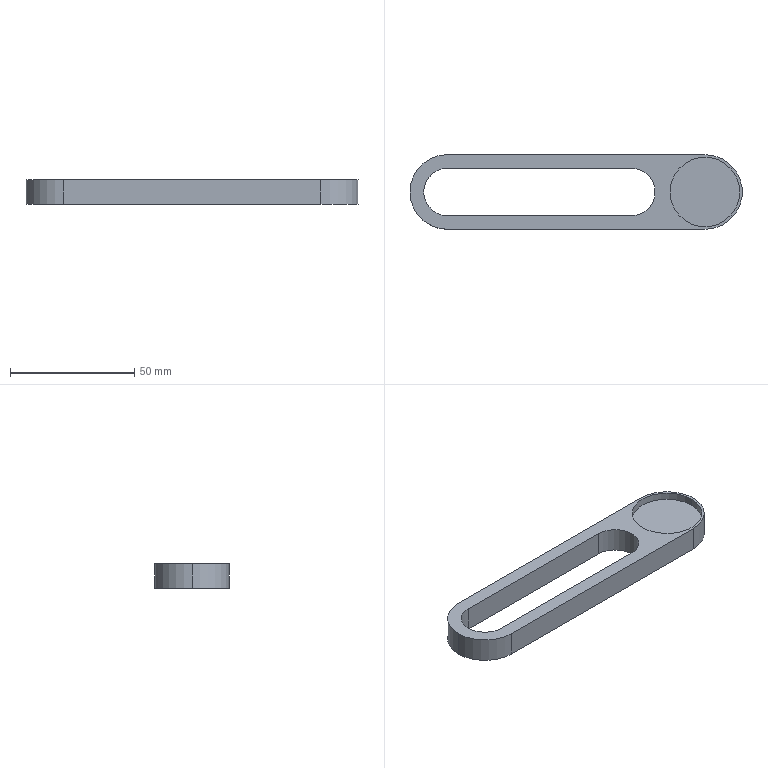Part | STEP file | PN_0040 | 1 solid | 15 faces | box 133.5 x 30 x 10 mm | volume 19376 mm3 | cylinder 8 | plane 7 | commonest cylinder face diameters 19 x3 30 x3 28 x2
STEP:
#1=CARTESIAN_POINT('',(0.,0.,0.));
#2=DIRECTION('',(0.,0.,1.));
#3=DIRECTION('',(1.,0.,0.));
#4=AXIS2_PLACEMENT_3D('',#1,#2,#3);
#5=CARTESIAN_POINT('',(117.5,0.,7.));
#6=VERTEX_POINT('',#5);
#7=CARTESIAN_POINT('',(117.5,0.,10.));
#8=VERTEX_POINT('',#7);
#9=CARTESIAN_POINT('',(117.5,0.,7.));
#10=DIRECTION('',(0.,0.,1.));
#11=VECTOR('',#10,1.);
#12=LINE('',#9,#11);
#13=CARTESIAN_POINT('',(103.5,0.,7.));
#14=DIRECTION('',(0.,0.,1.));
#15=DIRECTION('',(1.,0.,0.));
#16=AXIS2_PLACEMENT_3D('',#13,#14,#15);
#17=CYLINDRICAL_SURFACE('',#16,14.);
#18=CARTESIAN_POINT('',(6.283,0.));
#19=DIRECTION('',(0.,1.));
#20=VECTOR('',#19,1.);
#21=LINE('',#18,#20);
#22=(GEOMETRIC_REPRESENTATION_CONTEXT(2)PARAMETRIC_REPRESENTATION_CONTEXT()REPRESENTATION_CONTEXT('',''));
#23=DEFINITIONAL_REPRESENTATION('',(#21),#22);
#24=PCURVE('',#17,#23);
#25=CARTESIAN_POINT('',(103.5,0.,7.));
#26=DIRECTION('',(0.,0.,1.));
#27=DIRECTION('',(1.,0.,0.));
#28=AXIS2_PLACEMENT_3D('',#25,#26,#27);
#29=CYLINDRICAL_SURFACE('',#28,14.);
#30=CARTESIAN_POINT('',(0.,0.));
#31=DIRECTION('',(0.,1.));
#32=VECTOR('',#31,1.);
#33=LINE('',#30,#32);
#34=(GEOMETRIC_REPRESENTATION_CONTEXT(2)PARAMETRIC_REPRESENTATION_CONTEXT()REPRESENTATION_CONTEXT('',''));
#35=DEFINITIONAL_REPRESENTATION('',(#33),#34);
#36=PCURVE('',#29,#35);
#37=SURFACE_CURVE('',#12,(#24,#36),.PCURVE_S1.);
#38=EDGE_CURVE('',#6,#8,#37,.T.);
#39=ORIENTED_EDGE('',*,*,#38,.T.);
#40=CARTESIAN_POINT('',(89.5,0.,10.));
#41=VERTEX_POINT('',#40);
#42=CARTESIAN_POINT('',(103.5,0.,10.));
#43=DIRECTION('',(0.,0.,1.));
#44=DIRECTION('',(1.,0.,0.));
#45=AXIS2_PLACEMENT_3D('',#42,#43,#44);
#46=CIRCLE('',#45,14.);
#47=CARTESIAN_POINT('',(0.,3.));
#48=DIRECTION('',(1.,0.));
#49=VECTOR('',#48,1.);
#50=LINE('',#47,#49);
#51=(GEOMETRIC_REPRESENTATION_CONTEXT(2)PARAMETRIC_REPRESENTATION_CONTEXT()REPRESENTATION_CONTEXT('',''));
#52=DEFINITIONAL_REPRESENTATION('',(#50),#51);
#53=PCURVE('',#17,#52);
#54=CARTESIAN_POINT('',(0.,0.,10.));
#55=DIRECTION('',(0.,0.,1.));
#56=DIRECTION('',(1.,0.,0.));
#57=AXIS2_PLACEMENT_3D('',#54,#55,#56);
#58=PLANE('',#57);
#59=CARTESIAN_POINT('',(103.5,0.));
#60=DIRECTION('',(1.,0.));
#61=AXIS2_PLACEMENT_2D('',#59,#60);
#62=CIRCLE('',#61,14.);
#63=(GEOMETRIC_REPRESENTATION_CONTEXT(2)PARAMETRIC_REPRESENTATION_CONTEXT()REPRESENTATION_CONTEXT('',''));
#64=DEFINITIONAL_REPRESENTATION('',(#62),#63);
#65=PCURVE('',#58,#64);
#66=SURFACE_CURVE('',#46,(#53,#65),.PCURVE_S1.);
#67=EDGE_CURVE('',#41,#8,#66,.T.);
#68=ORIENTED_EDGE('',*,*,#67,.F.);
#69=CARTESIAN_POINT('',(89.5,0.,7.));
#70=VERTEX_POINT('',#69);
#71=CARTESIAN_POINT('',(89.5,0.,7.));
#72=DIRECTION('',(0.,0.,1.));
#73=VECTOR('',#72,1.);
#74=LINE('',#71,#73);
#75=CARTESIAN_POINT('',(3.142,0.));
#76=DIRECTION('',(0.,1.));
#77=VECTOR('',#76,1.);
#78=LINE('',#75,#77);
#79=(GEOMETRIC_REPRESENTATION_CONTEXT(2)PARAMETRIC_REPRESENTATION_CONTEXT()REPRESENTATION_CONTEXT('',''));
#80=DEFINITIONAL_REPRESENTATION('',(#78),#79);
#81=PCURVE('',#17,#80);
#82=CARTESIAN_POINT('',(3.142,0.));
#83=DIRECTION('',(0.,1.));
#84=VECTOR('',#83,1.);
#85=LINE('',#82,#84);
#86=(GEOMETRIC_REPRESENTATION_CONTEXT(2)PARAMETRIC_REPRESENTATION_CONTEXT()REPRESENTATION_CONTEXT('',''));
#87=DEFINITIONAL_REPRESENTATION('',(#85),#86);
#88=PCURVE('',#29,#87);
#89=SURFACE_CURVE('',#74,(#81,#88),.PCURVE_S1.);
#90=EDGE_CURVE('',#70,#41,#89,.T.);
#91=ORIENTED_EDGE('',*,*,#90,.F.);
#92=CARTESIAN_POINT('',(103.5,0.,7.));
#93=DIRECTION('',(0.,0.,1.));
#94=DIRECTION('',(1.,0.,0.));
#95=AXIS2_PLACEMENT_3D('',#92,#93,#94);
#96=CIRCLE('',#95,14.);
#97=CARTESIAN_POINT('',(0.,0.));
#98=DIRECTION('',(1.,0.));
#99=VECTOR('',#98,1.);
#100=LINE('',#97,#99);
#101=(GEOMETRIC_REPRESENTATION_CONTEXT(2)PARAMETRIC_REPRESENTATION_CONTEXT()REPRESENTATION_CONTEXT('',''));
#102=DEFINITIONAL_REPRESENTATION('',(#100),#101);
#103=PCURVE('',#17,#102);
#104=CARTESIAN_POINT('',(103.5,0.,7.));
#105=DIRECTION('',(0.,0.,1.));
#106=DIRECTION('',(1.,0.,0.));
#107=AXIS2_PLACEMENT_3D('',#104,#105,#106);
#108=PLANE('',#107);
#109=CARTESIAN_POINT('',(0.,0.));
#110=DIRECTION('',(1.,0.));
#111=AXIS2_PLACEMENT_2D('',#109,#110);
#112=CIRCLE('',#111,14.);
#113=(GEOMETRIC_REPRESENTATION_CONTEXT(2)PARAMETRIC_REPRESENTATION_CONTEXT()REPRESENTATION_CONTEXT('',''));
#114=DEFINITIONAL_REPRESENTATION('',(#112),#113);
#115=PCURVE('',#108,#114);
#116=SURFACE_CURVE('',#96,(#103,#115),.PCURVE_S1.);
#117=EDGE_CURVE('',#70,#6,#116,.T.);
#118=ORIENTED_EDGE('',*,*,#117,.T.);
#119=EDGE_LOOP('',(#39,#68,#91,#118));
#120=FACE_BOUND('',#119,.F.);
#121=ADVANCED_FACE('',(#120),#17,.F.);
#122=CARTESIAN_POINT('',(0.,9.5,10.));
#123=VERTEX_POINT('',#122);
#124=CARTESIAN_POINT('',(0.,9.5,0.));
#125=VERTEX_POINT('',#124);
#126=CARTESIAN_POINT('',(0.,9.5,10.));
#127=DIRECTION('',(0.,0.,-1.));
#128=VECTOR('',#127,1.);
#129=LINE('',#126,#128);
#130=CARTESIAN_POINT('',(0.,0.,10.));
#131=DIRECTION('',(0.,0.,-1.));
#132=DIRECTION('',(-1.,0.,0.));
#133=AXIS2_PLACEMENT_3D('',#130,#131,#132);
#134=CYLINDRICAL_SURFACE('',#133,9.5);
#135=CARTESIAN_POINT('',(1.571,0.));
#136=DIRECTION('',(0.,1.));
#137=VECTOR('',#136,1.);
#138=LINE('',#135,#137);
#139=(GEOMETRIC_REPRESENTATION_CONTEXT(2)PARAMETRIC_REPRESENTATION_CONTEXT()REPRESENTATION_CONTEXT('',''));
#140=DEFINITIONAL_REPRESENTATION('',(#138),#139);
#141=PCURVE('',#134,#140);
#142=CARTESIAN_POINT('',(0.,9.5,10.));
#143=DIRECTION('',(0.,-1.,0.));
#144=DIRECTION('',(0.,0.,-1.));
#145=AXIS2_PLACEMENT_3D('',#142,#143,#144);
#146=PLANE('',#145);
#147=CARTESIAN_POINT('',(0.,0.));
#148=DIRECTION('',(1.,0.));
#149=VECTOR('',#148,1.);
#150=LINE('',#147,#149);
#151=(GEOMETRIC_REPRESENTATION_CONTEXT(2)PARAMETRIC_REPRESENTATION_CONTEXT()REPRESENTATION_CONTEXT('',''));
#152=DEFINITIONAL_REPRESENTATION('',(#150),#151);
#153=PCURVE('',#146,#152);
#154=SURFACE_CURVE('',#129,(#141,#153),.PCURVE_S1.);
#155=EDGE_CURVE('',#123,#125,#154,.T.);
#156=ORIENTED_EDGE('',*,*,#155,.T.);
#157=CARTESIAN_POINT('',(-9.5,0.,0.));
#158=VERTEX_POINT('',#157);
#159=CARTESIAN_POINT('',(0.,0.,0.));
#160=DIRECTION('',(0.,0.,1.));
#161=DIRECTION('',(1.,0.,0.));
#162=AXIS2_PLACEMENT_3D('',#159,#160,#161);
#163=CIRCLE('',#162,9.5);
#164=CARTESIAN_POINT('',(3.142,10.));
#165=DIRECTION('',(-1.,0.));
#166=VECTOR('',#165,1.);
#167=LINE('',#164,#166);
#168=(GEOMETRIC_REPRESENTATION_CONTEXT(2)PARAMETRIC_REPRESENTATION_CONTEXT()REPRESENTATION_CONTEXT('',''));
#169=DEFINITIONAL_REPRESENTATION('',(#167),#168);
#170=PCURVE('',#134,#169);
#171=CARTESIAN_POINT('',(0.,0.,0.));
#172=DIRECTION('',(0.,0.,1.));
#173=DIRECTION('',(1.,0.,0.));
#174=AXIS2_PLACEMENT_3D('',#171,#172,#173);
#175=PLANE('',#174);
#176=CARTESIAN_POINT('',(0.,0.));
#177=DIRECTION('',(1.,0.));
#178=AXIS2_PLACEMENT_2D('',#176,#177);
#179=CIRCLE('',#178,9.5);
#180=(GEOMETRIC_REPRESENTATION_CONTEXT(2)PARAMETRIC_REPRESENTATION_CONTEXT()REPRESENTATION_CONTEXT('',''));
#181=DEFINITIONAL_REPRESENTATION('',(#179),#180);
#182=PCURVE('',#175,#181);
#183=SURFACE_CURVE('',#163,(#170,#182),.PCURVE_S1.);
#184=EDGE_CURVE('',#125,#158,#183,.T.);
#185=ORIENTED_EDGE('',*,*,#184,.T.);
#186=CARTESIAN_POINT('',(-9.5,0.,10.));
#187=VERTEX_POINT('',#186);
#188=CARTESIAN_POINT('',(-9.5,0.,10.));
#189=DIRECTION('',(0.,0.,-1.));
#190=VECTOR('',#189,1.);
#191=LINE('',#188,#190);
#192=CARTESIAN_POINT('',(0.,0.));
#193=DIRECTION('',(0.,1.));
#194=VECTOR('',#193,1.);
#195=LINE('',#192,#194);
#196=(GEOMETRIC_REPRESENTATION_CONTEXT(2)PARAMETRIC_REPRESENTATION_CONTEXT()REPRESENTATION_CONTEXT('',''));
#197=DEFINITIONAL_REPRESENTATION('',(#195),#196);
#198=PCURVE('',#134,#197);
#199=CARTESIAN_POINT('',(0.,0.,10.));
#200=DIRECTION('',(0.,0.,-1.));
#201=DIRECTION('',(-1.,0.,0.));
#202=AXIS2_PLACEMENT_3D('',#199,#200,#201);
#203=CYLINDRICAL_SURFACE('',#202,9.5);
#204=CARTESIAN_POINT('',(6.283,0.));
#205=DIRECTION('',(0.,1.));
#206=VECTOR('',#205,1.);
#207=LINE('',#204,#206);
#208=(GEOMETRIC_REPRESENTATION_CONTEXT(2)PARAMETRIC_REPRESENTATION_CONTEXT()REPRESENTATION_CONTEXT('',''));
#209=DEFINITIONAL_REPRESENTATION('',(#207),#208);
#210=PCURVE('',#203,#209);
#211=SURFACE_CURVE('',#191,(#198,#210),.PCURVE_S1.);
#212=EDGE_CURVE('',#187,#158,#211,.T.);
#213=ORIENTED_EDGE('',*,*,#212,.F.);
#214=CARTESIAN_POINT('',(0.,0.,10.));
#215=DIRECTION('',(0.,0.,1.));
#216=DIRECTION('',(1.,0.,0.));
#217=AXIS2_PLACEMENT_3D('',#214,#215,#216);
#218=CIRCLE('',#217,9.5);
#219=CARTESIAN_POINT('',(3.142,0.));
#220=DIRECTION('',(-1.,0.));
#221=VECTOR('',#220,1.);
#222=LINE('',#219,#221);
#223=(GEOMETRIC_REPRESENTATION_CONTEXT(2)PARAMETRIC_REPRESENTATION_CONTEXT()REPRESENTATION_CONTEXT('',''));
#224=DEFINITIONAL_REPRESENTATION('',(#222),#223);
#225=PCURVE('',#134,#224);
#226=CARTESIAN_POINT('',(0.,0.));
#227=DIRECTION('',(1.,0.));
#228=AXIS2_PLACEMENT_2D('',#226,#227);
#229=CIRCLE('',#228,9.5);
#230=(GEOMETRIC_REPRESENTATION_CONTEXT(2)PARAMETRIC_REPRESENTATION_CONTEXT()REPRESENTATION_CONTEXT('',''));
#231=DEFINITIONAL_REPRESENTATION('',(#229),#230);
#232=PCURVE('',#58,#231);
#233=SURFACE_CURVE('',#218,(#225,#232),.PCURVE_S1.);
#234=EDGE_CURVE('',#123,#187,#233,.T.);
#235=ORIENTED_EDGE('',*,*,#234,.F.);
#236=EDGE_LOOP('',(#156,#185,#213,#235));
#237=FACE_BOUND('',#236,.F.);
#238=ADVANCED_FACE('',(#237),#134,.F.);
#239=CARTESIAN_POINT('',(-15.,0.,10.));
#240=VERTEX_POINT('',#239);
#241=CARTESIAN_POINT('',(0.,-15.,10.));
#242=VERTEX_POINT('',#241);
#243=CARTESIAN_POINT('',(0.,0.,10.));
#244=DIRECTION('',(0.,0.,1.));
#245=DIRECTION('',(1.,0.,0.));
#246=AXIS2_PLACEMENT_3D('',#243,#244,#245);
#247=CIRCLE('',#246,15.);
#248=CARTESIAN_POINT('',(0.,0.,10.));
#249=DIRECTION('',(0.,0.,-1.));
#250=DIRECTION('',(-1.,0.,0.));
#251=AXIS2_PLACEMENT_3D('',#248,#249,#250);
#252=CYLINDRICAL_SURFACE('',#251,15.);
#253=CARTESIAN_POINT('',(9.425,0.));
#254=DIRECTION('',(-1.,0.));
#255=VECTOR('',#254,1.);
#256=LINE('',#253,#255);
#257=(GEOMETRIC_REPRESENTATION_CONTEXT(2)PARAMETRIC_REPRESENTATION_CONTEXT()REPRESENTATION_CONTEXT('',''));
#258=DEFINITIONAL_REPRESENTATION('',(#256),#257);
#259=PCURVE('',#252,#258);
#260=CARTESIAN_POINT('',(0.,0.));
#261=DIRECTION('',(1.,0.));
#262=AXIS2_PLACEMENT_2D('',#260,#261);
#263=CIRCLE('',#262,15.);
#264=(GEOMETRIC_REPRESENTATION_CONTEXT(2)PARAMETRIC_REPRESENTATION_CONTEXT()REPRESENTATION_CONTEXT('',''));
#265=DEFINITIONAL_REPRESENTATION('',(#263),#264);
#266=PCURVE('',#58,#265);
#267=SURFACE_CURVE('',#247,(#259,#266),.PCURVE_S1.);
#268=EDGE_CURVE('',#240,#242,#267,.T.);
#269=ORIENTED_EDGE('',*,*,#268,.F.);
#270=CARTESIAN_POINT('',(-15.,0.,0.));
#271=VERTEX_POINT('',#270);
#272=CARTESIAN_POINT('',(-15.,0.,10.));
#273=DIRECTION('',(0.,0.,-1.));
#274=VECTOR('',#273,1.);
#275=LINE('',#272,#274);
#276=CARTESIAN_POINT('',(6.283,0.));
#277=DIRECTION('',(0.,1.));
#278=VECTOR('',#277,1.);
#279=LINE('',#276,#278);
#280=(GEOMETRIC_REPRESENTATION_CONTEXT(2)PARAMETRIC_REPRESENTATION_CONTEXT()REPRESENTATION_CONTEXT('',''));
#281=DEFINITIONAL_REPRESENTATION('',(#279),#280);
#282=PCURVE('',#252,#281);
#283=CARTESIAN_POINT('',(0.,0.,10.));
#284=DIRECTION('',(0.,0.,-1.));
#285=DIRECTION('',(-1.,0.,0.));
#286=AXIS2_PLACEMENT_3D('',#283,#284,#285);
#287=CYLINDRICAL_SURFACE('',#286,15.);
#288=CARTESIAN_POINT('',(0.,0.));
#289=DIRECTION('',(0.,1.));
#290=VECTOR('',#289,1.);
#291=LINE('',#288,#290);
#292=(GEOMETRIC_REPRESENTATION_CONTEXT(2)PARAMETRIC_REPRESENTATION_CONTEXT()REPRESENTATION_CONTEXT('',''));
#293=DEFINITIONAL_REPRESENTATION('',(#291),#292);
#294=PCURVE('',#287,#293);
#295=SURFACE_CURVE('',#275,(#282,#294),.PCURVE_S1.);
#296=EDGE_CURVE('',#240,#271,#295,.T.);
#297=ORIENTED_EDGE('',*,*,#296,.T.);
#298=CARTESIAN_POINT('',(0.,-15.,0.));
#299=VERTEX_POINT('',#298);
#300=CARTESIAN_POINT('',(0.,0.,0.));
#301=DIRECTION('',(0.,0.,1.));
#302=DIRECTION('',(1.,0.,0.));
#303=AXIS2_PLACEMENT_3D('',#300,#301,#302);
#304=CIRCLE('',#303,15.);
#305=CARTESIAN_POINT('',(9.425,10.));
#306=DIRECTION('',(-1.,0.));
#307=VECTOR('',#306,1.);
#308=LINE('',#305,#307);
#309=(GEOMETRIC_REPRESENTATION_CONTEXT(2)PARAMETRIC_REPRESENTATION_CONTEXT()REPRESENTATION_CONTEXT('',''));
#310=DEFINITIONAL_REPRESENTATION('',(#308),#309);
#311=PCURVE('',#252,#310);
#312=CARTESIAN_POINT('',(0.,0.));
#313=DIRECTION('',(1.,0.));
#314=AXIS2_PLACEMENT_2D('',#312,#313);
#315=CIRCLE('',#314,15.);
#316=(GEOMETRIC_REPRESENTATION_CONTEXT(2)PARAMETRIC_REPRESENTATION_CONTEXT()REPRESENTATION_CONTEXT('',''));
#317=DEFINITIONAL_REPRESENTATION('',(#315),#316);
#318=PCURVE('',#175,#317);
#319=SURFACE_CURVE('',#304,(#311,#318),.PCURVE_S1.);
#320=EDGE_CURVE('',#271,#299,#319,.T.);
#321=ORIENTED_EDGE('',*,*,#320,.T.);
#322=CARTESIAN_POINT('',(0.,-15.,10.));
#323=DIRECTION('',(0.,0.,-1.));
#324=VECTOR('',#323,1.);
#325=LINE('',#322,#324);
#326=CARTESIAN_POINT('',(4.712,0.));
#327=DIRECTION('',(0.,1.));
#328=VECTOR('',#327,1.);
#329=LINE('',#326,#328);
#330=(GEOMETRIC_REPRESENTATION_CONTEXT(2)PARAMETRIC_REPRESENTATION_CONTEXT()REPRESENTATION_CONTEXT('',''));
#331=DEFINITIONAL_REPRESENTATION('',(#329),#330);
#332=PCURVE('',#252,#331);
#333=CARTESIAN_POINT('',(0.,-15.,10.));
#334=DIRECTION('',(0.,1.,0.));
#335=DIRECTION('',(-1.,0.,0.));
#336=AXIS2_PLACEMENT_3D('',#333,#334,#335);
#337=PLANE('',#336);
#338=CARTESIAN_POINT('',(0.,0.));
#339=DIRECTION('',(0.,-1.));
#340=VECTOR('',#339,1.);
#341=LINE('',#338,#340);
#342=(GEOMETRIC_REPRESENTATION_CONTEXT(2)PARAMETRIC_REPRESENTATION_CONTEXT()REPRESENTATION_CONTEXT('',''));
#343=DEFINITIONAL_REPRESENTATION('',(#341),#342);
#344=PCURVE('',#337,#343);
#345=SURFACE_CURVE('',#325,(#332,#344),.PCURVE_S1.);
#346=EDGE_CURVE('',#242,#299,#345,.T.);
#347=ORIENTED_EDGE('',*,*,#346,.F.);
#348=EDGE_LOOP('',(#269,#297,#321,#347));
#349=FACE_BOUND('',#348,.T.);
#350=ADVANCED_FACE('',(#349),#252,.T.);
#351=CARTESIAN_POINT('',(103.5,0.,10.));
#352=DIRECTION('',(0.,0.,1.));
#353=DIRECTION('',(1.,0.,0.));
#354=AXIS2_PLACEMENT_3D('',#351,#352,#353);
#355=CIRCLE('',#354,14.);
#356=CARTESIAN_POINT('',(103.5,0.));
#357=DIRECTION('',(1.,0.));
#358=AXIS2_PLACEMENT_2D('',#356,#357);
#359=CIRCLE('',#358,14.);
#360=(GEOMETRIC_REPRESENTATION_CONTEXT(2)PARAMETRIC_REPRESENTATION_CONTEXT()REPRESENTATION_CONTEXT('',''));
#361=DEFINITIONAL_REPRESENTATION('',(#359),#360);
#362=PCURVE('',#58,#361);
#363=CARTESIAN_POINT('',(0.,3.));
#364=DIRECTION('',(1.,0.));
#365=VECTOR('',#364,1.);
#366=LINE('',#363,#365);
#367=(GEOMETRIC_REPRESENTATION_CONTEXT(2)PARAMETRIC_REPRESENTATION_CONTEXT()REPRESENTATION_CONTEXT('',''));
#368=DEFINITIONAL_REPRESENTATION('',(#366),#367);
#369=PCURVE('',#29,#368);
#370=SURFACE_CURVE('',#355,(#362,#369),.PCURVE_S1.);
#371=EDGE_CURVE('',#8,#41,#370,.T.);
#372=ORIENTED_EDGE('',*,*,#371,.F.);
#373=ORIENTED_EDGE('',*,*,#67,.F.);
#374=EDGE_LOOP('',(#372,#373));
#375=FACE_BOUND('',#374,.T.);
#376=CARTESIAN_POINT('',(0.,15.,10.));
#377=VERTEX_POINT('',#376);
#378=CARTESIAN_POINT('',(0.,0.,10.));
#379=DIRECTION('',(0.,0.,1.));
#380=DIRECTION('',(1.,0.,0.));
#381=AXIS2_PLACEMENT_3D('',#378,#379,#380);
#382=CIRCLE('',#381,15.);
#383=CARTESIAN_POINT('',(0.,0.));
#384=DIRECTION('',(1.,0.));
#385=AXIS2_PLACEMENT_2D('',#383,#384);
#386=CIRCLE('',#385,15.);
#387=(GEOMETRIC_REPRESENTATION_CONTEXT(2)PARAMETRIC_REPRESENTATION_CONTEXT()REPRESENTATION_CONTEXT('',''));
#388=DEFINITIONAL_REPRESENTATION('',(#386),#387);
#389=PCURVE('',#58,#388);
#390=CARTESIAN_POINT('',(3.142,0.));
#391=DIRECTION('',(-1.,0.));
#392=VECTOR('',#391,1.);
#393=LINE('',#390,#392);
#394=(GEOMETRIC_REPRESENTATION_CONTEXT(2)PARAMETRIC_REPRESENTATION_CONTEXT()REPRESENTATION_CONTEXT('',''));
#395=DEFINITIONAL_REPRESENTATION('',(#393),#394);
#396=PCURVE('',#287,#395);
#397=SURFACE_CURVE('',#382,(#389,#396),.PCURVE_S1.);
#398=EDGE_CURVE('',#377,#240,#397,.T.);
#399=ORIENTED_EDGE('',*,*,#398,.T.);
#400=ORIENTED_EDGE('',*,*,#268,.T.);
#401=CARTESIAN_POINT('',(103.5,-15.,10.));
#402=VERTEX_POINT('',#401);
#403=CARTESIAN_POINT('',(0.,-15.,10.));
#404=DIRECTION('',(1.,0.,0.));
#405=VECTOR('',#404,1.);
#406=LINE('',#403,#405);
#407=CARTESIAN_POINT('',(0.,-15.));
#408=DIRECTION('',(1.,0.));
#409=VECTOR('',#408,1.);
#410=LINE('',#407,#409);
#411=(GEOMETRIC_REPRESENTATION_CONTEXT(2)PARAMETRIC_REPRESENTATION_CONTEXT()REPRESENTATION_CONTEXT('',''));
#412=DEFINITIONAL_REPRESENTATION('',(#410),#411);
#413=PCURVE('',#58,#412);
#414=CARTESIAN_POINT('',(0.,0.));
#415=DIRECTION('',(-1.,0.));
#416=VECTOR('',#415,1.);
#417=LINE('',#414,#416);
#418=(GEOMETRIC_REPRESENTATION_CONTEXT(2)PARAMETRIC_REPRESENTATION_CONTEXT()REPRESENTATION_CONTEXT('',''));
#419=DEFINITIONAL_REPRESENTATION('',(#417),#418);
#420=PCURVE('',#337,#419);
#421=SURFACE_CURVE('',#406,(#413,#420),.PCURVE_S1.);
#422=EDGE_CURVE('',#242,#402,#421,.T.);
#423=ORIENTED_EDGE('',*,*,#422,.T.);
#424=CARTESIAN_POINT('',(103.5,15.,10.));
#425=VERTEX_POINT('',#424);
#426=CARTESIAN_POINT('',(103.5,0.,10.));
#427=DIRECTION('',(0.,0.,1.));
#428=DIRECTION('',(1.,0.,0.));
#429=AXIS2_PLACEMENT_3D('',#426,#427,#428);
#430=CIRCLE('',#429,15.);
#431=CARTESIAN_POINT('',(103.5,0.));
#432=DIRECTION('',(1.,0.));
#433=AXIS2_PLACEMENT_2D('',#431,#432);
#434=CIRCLE('',#433,15.);
#435=(GEOMETRIC_REPRESENTATION_CONTEXT(2)PARAMETRIC_REPRESENTATION_CONTEXT()REPRESENTATION_CONTEXT('',''));
#436=DEFINITIONAL_REPRESENTATION('',(#434),#435);
#437=PCURVE('',#58,#436);
#438=CARTESIAN_POINT('',(103.5,0.,10.));
#439=DIRECTION('',(0.,0.,-1.));
#440=DIRECTION('',(-1.,0.,0.));
#441=AXIS2_PLACEMENT_3D('',#438,#439,#440);
#442=CYLINDRICAL_SURFACE('',#441,15.);
#443=CARTESIAN_POINT('',(9.425,0.));
#444=DIRECTION('',(-1.,0.));
#445=VECTOR('',#444,1.);
#446=LINE('',#443,#445);
#447=(GEOMETRIC_REPRESENTATION_CONTEXT(2)PARAMETRIC_REPRESENTATION_CONTEXT()REPRESENTATION_CONTEXT('',''));
#448=DEFINITIONAL_REPRESENTATION('',(#446),#447);
#449=PCURVE('',#442,#448);
#450=SURFACE_CURVE('',#430,(#437,#449),.PCURVE_S1.);
#451=EDGE_CURVE('',#402,#425,#450,.T.);
#452=ORIENTED_EDGE('',*,*,#451,.T.);
#453=CARTESIAN_POINT('',(0.,15.,10.));
#454=DIRECTION('',(-1.,0.,0.));
#455=VECTOR('',#454,1.);
#456=LINE('',#453,#455);
#457=CARTESIAN_POINT('',(0.,15.));
#458=DIRECTION('',(-1.,0.));
#459=VECTOR('',#458,1.);
#460=LINE('',#457,#459);
#461=(GEOMETRIC_REPRESENTATION_CONTEXT(2)PARAMETRIC_REPRESENTATION_CONTEXT()REPRESENTATION_CONTEXT('',''));
#462=DEFINITIONAL_REPRESENTATION('',(#460),#461);
#463=PCURVE('',#58,#462);
#464=CARTESIAN_POINT('',(0.,15.,10.));
#465=DIRECTION('',(0.,-1.,0.));
#466=DIRECTION('',(0.,0.,-1.));
#467=AXIS2_PLACEMENT_3D('',#464,#465,#466);
#468=PLANE('',#467);
#469=CARTESIAN_POINT('',(0.,0.));
#470=DIRECTION('',(0.,-1.));
#471=VECTOR('',#470,1.);
#472=LINE('',#469,#471);
#473=(GEOMETRIC_REPRESENTATION_CONTEXT(2)PARAMETRIC_REPRESENTATION_CONTEXT()REPRESENTATION_CONTEXT('',''));
#474=DEFINITIONAL_REPRESENTATION('',(#472),#473);
#475=PCURVE('',#468,#474);
#476=SURFACE_CURVE('',#456,(#463,#475),.PCURVE_S1.);
#477=EDGE_CURVE('',#425,#377,#476,.T.);
#478=ORIENTED_EDGE('',*,*,#477,.T.);
#479=EDGE_LOOP('',(#399,#400,#423,#452,#478));
#480=FACE_BOUND('',#479,.T.);
#481=CARTESIAN_POINT('',(0.,-9.5,10.));
#482=VERTEX_POINT('',#481);
#483=CARTESIAN_POINT('',(74.,-9.5,10.));
#484=VERTEX_POINT('',#483);
#485=CARTESIAN_POINT('',(0.,-9.5,10.));
#486=DIRECTION('',(1.,0.,0.));
#487=VECTOR('',#486,1.);
#488=LINE('',#485,#487);
#489=CARTESIAN_POINT('',(0.,-9.5));
#490=DIRECTION('',(1.,0.));
#491=VECTOR('',#490,1.);
#492=LINE('',#489,#491);
#493=(GEOMETRIC_REPRESENTATION_CONTEXT(2)PARAMETRIC_REPRESENTATION_CONTEXT()REPRESENTATION_CONTEXT('',''));
#494=DEFINITIONAL_REPRESENTATION('',(#492),#493);
#495=PCURVE('',#58,#494);
#496=CARTESIAN_POINT('',(0.,-9.5,10.));
#497=DIRECTION('',(0.,1.,0.));
#498=DIRECTION('',(-1.,0.,0.));
#499=AXIS2_PLACEMENT_3D('',#496,#497,#498);
#500=PLANE('',#499);
#501=CARTESIAN_POINT('',(0.,0.));
#502=DIRECTION('',(-1.,0.));
#503=VECTOR('',#502,1.);
#504=LINE('',#501,#503);
#505=(GEOMETRIC_REPRESENTATION_CONTEXT(2)PARAMETRIC_REPRESENTATION_CONTEXT()REPRESENTATION_CONTEXT('',''));
#506=DEFINITIONAL_REPRESENTATION('',(#504),#505);
#507=PCURVE('',#500,#506);
#508=SURFACE_CURVE('',#488,(#495,#507),.PCURVE_S1.);
#509=EDGE_CURVE('',#482,#484,#508,.T.);
#510=ORIENTED_EDGE('',*,*,#509,.F.);
#511=CARTESIAN_POINT('',(0.,0.,10.));
#512=DIRECTION('',(0.,0.,1.));
#513=DIRECTION('',(1.,0.,0.));
#514=AXIS2_PLACEMENT_3D('',#511,#512,#513);
#515=CIRCLE('',#514,9.5);
#516=CARTESIAN_POINT('',(0.,0.));
#517=DIRECTION('',(1.,0.));
#518=AXIS2_PLACEMENT_2D('',#516,#517);
#519=CIRCLE('',#518,9.5);
#520=(GEOMETRIC_REPRESENTATION_CONTEXT(2)PARAMETRIC_REPRESENTATION_CONTEXT()REPRESENTATION_CONTEXT('',''));
#521=DEFINITIONAL_REPRESENTATION('',(#519),#520);
#522=PCURVE('',#58,#521);
#523=CARTESIAN_POINT('',(9.425,0.));
#524=DIRECTION('',(-1.,0.));
#525=VECTOR('',#524,1.);
#526=LINE('',#523,#525);
#527=(GEOMETRIC_REPRESENTATION_CONTEXT(2)PARAMETRIC_REPRESENTATION_CONTEXT()REPRESENTATION_CONTEXT('',''));
#528=DEFINITIONAL_REPRESENTATION('',(#526),#527);
#529=PCURVE('',#203,#528);
#530=SURFACE_CURVE('',#515,(#522,#529),.PCURVE_S1.);
#531=EDGE_CURVE('',#187,#482,#530,.T.);
#532=ORIENTED_EDGE('',*,*,#531,.F.);
#533=ORIENTED_EDGE('',*,*,#234,.F.);
#534=CARTESIAN_POINT('',(74.,9.5,10.));
#535=VERTEX_POINT('',#534);
#536=CARTESIAN_POINT('',(0.,9.5,10.));
#537=DIRECTION('',(-1.,0.,0.));
#538=VECTOR('',#537,1.);
#539=LINE('',#536,#538);
#540=CARTESIAN_POINT('',(0.,9.5));
#541=DIRECTION('',(-1.,0.));
#542=VECTOR('',#541,1.);
#543=LINE('',#540,#542);
#544=(GEOMETRIC_REPRESENTATION_CONTEXT(2)PARAMETRIC_REPRESENTATION_CONTEXT()REPRESENTATION_CONTEXT('',''));
#545=DEFINITIONAL_REPRESENTATION('',(#543),#544);
#546=PCURVE('',#58,#545);
#547=CARTESIAN_POINT('',(0.,0.));
#548=DIRECTION('',(0.,-1.));
#549=VECTOR('',#548,1.);
#550=LINE('',#547,#549);
#551=(GEOMETRIC_REPRESENTATION_CONTEXT(2)PARAMETRIC_REPRESENTATION_CONTEXT()REPRESENTATION_CONTEXT('',''));
#552=DEFINITIONAL_REPRESENTATION('',(#550),#551);
#553=PCURVE('',#146,#552);
#554=SURFACE_CURVE('',#539,(#546,#553),.PCURVE_S1.);
#555=EDGE_CURVE('',#535,#123,#554,.T.);
#556=ORIENTED_EDGE('',*,*,#555,.F.);
#557=CARTESIAN_POINT('',(74.,0.,10.));
#558=DIRECTION('',(0.,0.,1.));
#559=DIRECTION('',(1.,0.,0.));
#560=AXIS2_PLACEMENT_3D('',#557,#558,#559);
#561=CIRCLE('',#560,9.5);
#562=CARTESIAN_POINT('',(74.,0.));
#563=DIRECTION('',(1.,0.));
#564=AXIS2_PLACEMENT_2D('',#562,#563);
#565=CIRCLE('',#564,9.5);
#566=(GEOMETRIC_REPRESENTATION_CONTEXT(2)PARAMETRIC_REPRESENTATION_CONTEXT()REPRESENTATION_CONTEXT('',''));
#567=DEFINITIONAL_REPRESENTATION('',(#565),#566);
#568=PCURVE('',#58,#567);
#569=CARTESIAN_POINT('',(74.,0.,10.));
#570=DIRECTION('',(0.,0.,-1.));
#571=DIRECTION('',(-1.,0.,0.));
#572=AXIS2_PLACEMENT_3D('',#569,#570,#571);
#573=CYLINDRICAL_SURFACE('',#572,9.5);
#574=CARTESIAN_POINT('',(9.425,0.));
#575=DIRECTION('',(-1.,0.));
#576=VECTOR('',#575,1.);
#577=LINE('',#574,#576);
#578=(GEOMETRIC_REPRESENTATION_CONTEXT(2)PARAMETRIC_REPRESENTATION_CONTEXT()REPRESENTATION_CONTEXT('',''));
#579=DEFINITIONAL_REPRESENTATION('',(#577),#578);
#580=PCURVE('',#573,#579);
#581=SURFACE_CURVE('',#561,(#568,#580),.PCURVE_S1.);
#582=EDGE_CURVE('',#484,#535,#581,.T.);
#583=ORIENTED_EDGE('',*,*,#582,.F.);
#584=EDGE_LOOP('',(#510,#532,#533,#556,#583));
#585=FACE_BOUND('',#584,.T.);
#586=ADVANCED_FACE('',(#375,#480,#585),#58,.T.);
#587=CARTESIAN_POINT('',(0.,15.,0.));
#588=VERTEX_POINT('',#587);
#589=CARTESIAN_POINT('',(0.,0.,0.));
#590=DIRECTION('',(0.,0.,1.));
#591=DIRECTION('',(1.,0.,0.));
#592=AXIS2_PLACEMENT_3D('',#589,#590,#591);
#593=CIRCLE('',#592,15.);
#594=CARTESIAN_POINT('',(0.,0.));
#595=DIRECTION('',(1.,0.));
#596=AXIS2_PLACEMENT_2D('',#594,#595);
#597=CIRCLE('',#596,15.);
#598=(GEOMETRIC_REPRESENTATION_CONTEXT(2)PARAMETRIC_REPRESENTATION_CONTEXT()REPRESENTATION_CONTEXT('',''));
#599=DEFINITIONAL_REPRESENTATION('',(#597),#598);
#600=PCURVE('',#175,#599);
#601=CARTESIAN_POINT('',(3.142,10.));
#602=DIRECTION('',(-1.,0.));
#603=VECTOR('',#602,1.);
#604=LINE('',#601,#603);
#605=(GEOMETRIC_REPRESENTATION_CONTEXT(2)PARAMETRIC_REPRESENTATION_CONTEXT()REPRESENTATION_CONTEXT('',''));
#606=DEFINITIONAL_REPRESENTATION('',(#604),#605);
#607=PCURVE('',#287,#606);
#608=SURFACE_CURVE('',#593,(#600,#607),.PCURVE_S1.);
#609=EDGE_CURVE('',#588,#271,#608,.T.);
#610=ORIENTED_EDGE('',*,*,#609,.F.);
#611=CARTESIAN_POINT('',(103.5,15.,0.));
#612=VERTEX_POINT('',#611);
#613=CARTESIAN_POINT('',(0.,15.,0.));
#614=DIRECTION('',(-1.,0.,0.));
#615=VECTOR('',#614,1.);
#616=LINE('',#613,#615);
#617=CARTESIAN_POINT('',(0.,15.));
#618=DIRECTION('',(-1.,0.));
#619=VECTOR('',#618,1.);
#620=LINE('',#617,#619);
#621=(GEOMETRIC_REPRESENTATION_CONTEXT(2)PARAMETRIC_REPRESENTATION_CONTEXT()REPRESENTATION_CONTEXT('',''));
#622=DEFINITIONAL_REPRESENTATION('',(#620),#621);
#623=PCURVE('',#175,#622);
#624=CARTESIAN_POINT('',(10.,0.));
#625=DIRECTION('',(0.,-1.));
#626=VECTOR('',#625,1.);
#627=LINE('',#624,#626);
#628=(GEOMETRIC_REPRESENTATION_CONTEXT(2)PARAMETRIC_REPRESENTATION_CONTEXT()REPRESENTATION_CONTEXT('',''));
#629=DEFINITIONAL_REPRESENTATION('',(#627),#628);
#630=PCURVE('',#468,#629);
#631=SURFACE_CURVE('',#616,(#623,#630),.PCURVE_S1.);
#632=EDGE_CURVE('',#612,#588,#631,.T.);
#633=ORIENTED_EDGE('',*,*,#632,.F.);
#634=CARTESIAN_POINT('',(103.5,-15.,0.));
#635=VERTEX_POINT('',#634);
#636=CARTESIAN_POINT('',(103.5,0.,0.));
#637=DIRECTION('',(0.,0.,1.));
#638=DIRECTION('',(1.,0.,0.));
#639=AXIS2_PLACEMENT_3D('',#636,#637,#638);
#640=CIRCLE('',#639,15.);
#641=CARTESIAN_POINT('',(103.5,0.));
#642=DIRECTION('',(1.,0.));
#643=AXIS2_PLACEMENT_2D('',#641,#642);
#644=CIRCLE('',#643,15.);
#645=(GEOMETRIC_REPRESENTATION_CONTEXT(2)PARAMETRIC_REPRESENTATION_CONTEXT()REPRESENTATION_CONTEXT('',''));
#646=DEFINITIONAL_REPRESENTATION('',(#644),#645);
#647=PCURVE('',#175,#646);
#648=CARTESIAN_POINT('',(9.425,10.));
#649=DIRECTION('',(-1.,0.));
#650=VECTOR('',#649,1.);
#651=LINE('',#648,#650);
#652=(GEOMETRIC_REPRESENTATION_CONTEXT(2)PARAMETRIC_REPRESENTATION_CONTEXT()REPRESENTATION_CONTEXT('',''));
#653=DEFINITIONAL_REPRESENTATION('',(#651),#652);
#654=PCURVE('',#442,#653);
#655=SURFACE_CURVE('',#640,(#647,#654),.PCURVE_S1.);
#656=EDGE_CURVE('',#635,#612,#655,.T.);
#657=ORIENTED_EDGE('',*,*,#656,.F.);
#658=CARTESIAN_POINT('',(0.,-15.,0.));
#659=DIRECTION('',(1.,0.,0.));
#660=VECTOR('',#659,1.);
#661=LINE('',#658,#660);
#662=CARTESIAN_POINT('',(0.,-15.));
#663=DIRECTION('',(1.,0.));
#664=VECTOR('',#663,1.);
#665=LINE('',#662,#664);
#666=(GEOMETRIC_REPRESENTATION_CONTEXT(2)PARAMETRIC_REPRESENTATION_CONTEXT()REPRESENTATION_CONTEXT('',''));
#667=DEFINITIONAL_REPRESENTATION('',(#665),#666);
#668=PCURVE('',#175,#667);
#669=CARTESIAN_POINT('',(0.,-10.));
#670=DIRECTION('',(-1.,0.));
#671=VECTOR('',#670,1.);
#672=LINE('',#669,#671);
#673=(GEOMETRIC_REPRESENTATION_CONTEXT(2)PARAMETRIC_REPRESENTATION_CONTEXT()REPRESENTATION_CONTEXT('',''));
#674=DEFINITIONAL_REPRESENTATION('',(#672),#673);
#675=PCURVE('',#337,#674);
#676=SURFACE_CURVE('',#661,(#668,#675),.PCURVE_S1.);
#677=EDGE_CURVE('',#299,#635,#676,.T.);
#678=ORIENTED_EDGE('',*,*,#677,.F.);
#679=ORIENTED_EDGE('',*,*,#320,.F.);
#680=EDGE_LOOP('',(#610,#633,#657,#678,#679));
#681=FACE_BOUND('',#680,.T.);
#682=ORIENTED_EDGE('',*,*,#184,.T.);
#683=CARTESIAN_POINT('',(0.,-9.5,0.));
#684=VERTEX_POINT('',#683);
#685=CARTESIAN_POINT('',(0.,0.,0.));
#686=DIRECTION('',(0.,0.,1.));
#687=DIRECTION('',(1.,0.,0.));
#688=AXIS2_PLACEMENT_3D('',#685,#686,#687);
#689=CIRCLE('',#688,9.5);
#690=CARTESIAN_POINT('',(0.,0.));
#691=DIRECTION('',(1.,0.));
#692=AXIS2_PLACEMENT_2D('',#690,#691);
#693=CIRCLE('',#692,9.5);
#694=(GEOMETRIC_REPRESENTATION_CONTEXT(2)PARAMETRIC_REPRESENTATION_CONTEXT()REPRESENTATION_CONTEXT('',''));
#695=DEFINITIONAL_REPRESENTATION('',(#693),#694);
#696=PCURVE('',#175,#695);
#697=CARTESIAN_POINT('',(9.425,10.));
#698=DIRECTION('',(-1.,0.));
#699=VECTOR('',#698,1.);
#700=LINE('',#697,#699);
#701=(GEOMETRIC_REPRESENTATION_CONTEXT(2)PARAMETRIC_REPRESENTATION_CONTEXT()REPRESENTATION_CONTEXT('',''));
#702=DEFINITIONAL_REPRESENTATION('',(#700),#701);
#703=PCURVE('',#203,#702);
#704=SURFACE_CURVE('',#689,(#696,#703),.PCURVE_S1.);
#705=EDGE_CURVE('',#158,#684,#704,.T.);
#706=ORIENTED_EDGE('',*,*,#705,.T.);
#707=CARTESIAN_POINT('',(74.,-9.5,0.));
#708=VERTEX_POINT('',#707);
#709=CARTESIAN_POINT('',(0.,-9.5,0.));
#710=DIRECTION('',(1.,0.,0.));
#711=VECTOR('',#710,1.);
#712=LINE('',#709,#711);
#713=CARTESIAN_POINT('',(0.,-9.5));
#714=DIRECTION('',(1.,0.));
#715=VECTOR('',#714,1.);
#716=LINE('',#713,#715);
#717=(GEOMETRIC_REPRESENTATION_CONTEXT(2)PARAMETRIC_REPRESENTATION_CONTEXT()REPRESENTATION_CONTEXT('',''));
#718=DEFINITIONAL_REPRESENTATION('',(#716),#717);
#719=PCURVE('',#175,#718);
#720=CARTESIAN_POINT('',(0.,-10.));
#721=DIRECTION('',(-1.,0.));
#722=VECTOR('',#721,1.);
#723=LINE('',#720,#722);
#724=(GEOMETRIC_REPRESENTATION_CONTEXT(2)PARAMETRIC_REPRESENTATION_CONTEXT()REPRESENTATION_CONTEXT('',''));
#725=DEFINITIONAL_REPRESENTATION('',(#723),#724);
#726=PCURVE('',#500,#725);
#727=SURFACE_CURVE('',#712,(#719,#726),.PCURVE_S1.);
#728=EDGE_CURVE('',#684,#708,#727,.T.);
#729=ORIENTED_EDGE('',*,*,#728,.T.);
#730=CARTESIAN_POINT('',(74.,9.5,0.));
#731=VERTEX_POINT('',#730);
#732=CARTESIAN_POINT('',(74.,0.,0.));
#733=DIRECTION('',(0.,0.,1.));
#734=DIRECTION('',(1.,0.,0.));
#735=AXIS2_PLACEMENT_3D('',#732,#733,#734);
#736=CIRCLE('',#735,9.5);
#737=CARTESIAN_POINT('',(74.,0.));
#738=DIRECTION('',(1.,0.));
#739=AXIS2_PLACEMENT_2D('',#737,#738);
#740=CIRCLE('',#739,9.5);
#741=(GEOMETRIC_REPRESENTATION_CONTEXT(2)PARAMETRIC_REPRESENTATION_CONTEXT()REPRESENTATION_CONTEXT('',''));
#742=DEFINITIONAL_REPRESENTATION('',(#740),#741);
#743=PCURVE('',#175,#742);
#744=CARTESIAN_POINT('',(9.425,10.));
#745=DIRECTION('',(-1.,0.));
#746=VECTOR('',#745,1.);
#747=LINE('',#744,#746);
#748=(GEOMETRIC_REPRESENTATION_CONTEXT(2)PARAMETRIC_REPRESENTATION_CONTEXT()REPRESENTATION_CONTEXT('',''));
#749=DEFINITIONAL_REPRESENTATION('',(#747),#748);
#750=PCURVE('',#573,#749);
#751=SURFACE_CURVE('',#736,(#743,#750),.PCURVE_S1.);
#752=EDGE_CURVE('',#708,#731,#751,.T.);
#753=ORIENTED_EDGE('',*,*,#752,.T.);
#754=CARTESIAN_POINT('',(0.,9.5,0.));
#755=DIRECTION('',(-1.,0.,0.));
#756=VECTOR('',#755,1.);
#757=LINE('',#754,#756);
#758=CARTESIAN_POINT('',(0.,9.5));
#759=DIRECTION('',(-1.,0.));
#760=VECTOR('',#759,1.);
#761=LINE('',#758,#760);
#762=(GEOMETRIC_REPRESENTATION_CONTEXT(2)PARAMETRIC_REPRESENTATION_CONTEXT()REPRESENTATION_CONTEXT('',''));
#763=DEFINITIONAL_REPRESENTATION('',(#761),#762);
#764=PCURVE('',#175,#763);
#765=CARTESIAN_POINT('',(10.,0.));
#766=DIRECTION('',(0.,-1.));
#767=VECTOR('',#766,1.);
#768=LINE('',#765,#767);
#769=(GEOMETRIC_REPRESENTATION_CONTEXT(2)PARAMETRIC_REPRESENTATION_CONTEXT()REPRESENTATION_CONTEXT('',''));
#770=DEFINITIONAL_REPRESENTATION('',(#768),#769);
#771=PCURVE('',#146,#770);
#772=SURFACE_CURVE('',#757,(#764,#771),.PCURVE_S1.);
#773=EDGE_CURVE('',#731,#125,#772,.T.);
#774=ORIENTED_EDGE('',*,*,#773,.T.);
#775=EDGE_LOOP('',(#682,#706,#729,#753,#774));
#776=FACE_BOUND('',#775,.T.);
#777=ADVANCED_FACE('',(#681,#776),#175,.F.);
#778=ORIENTED_EDGE('',*,*,#296,.F.);
#779=ORIENTED_EDGE('',*,*,#398,.F.);
#780=CARTESIAN_POINT('',(0.,15.,10.));
#781=DIRECTION('',(0.,0.,-1.));
#782=VECTOR('',#781,1.);
#783=LINE('',#780,#782);
#784=CARTESIAN_POINT('',(1.571,0.));
#785=DIRECTION('',(0.,1.));
#786=VECTOR('',#785,1.);
#787=LINE('',#784,#786);
#788=(GEOMETRIC_REPRESENTATION_CONTEXT(2)PARAMETRIC_REPRESENTATION_CONTEXT()REPRESENTATION_CONTEXT('',''));
#789=DEFINITIONAL_REPRESENTATION('',(#787),#788);
#790=PCURVE('',#287,#789);
#791=CARTESIAN_POINT('',(0.,0.));
#792=DIRECTION('',(1.,0.));
#793=VECTOR('',#792,1.);
#794=LINE('',#791,#793);
#795=(GEOMETRIC_REPRESENTATION_CONTEXT(2)PARAMETRIC_REPRESENTATION_CONTEXT()REPRESENTATION_CONTEXT('',''));
#796=DEFINITIONAL_REPRESENTATION('',(#794),#795);
#797=PCURVE('',#468,#796);
#798=SURFACE_CURVE('',#783,(#790,#797),.PCURVE_S1.);
#799=EDGE_CURVE('',#377,#588,#798,.T.);
#800=ORIENTED_EDGE('',*,*,#799,.T.);
#801=ORIENTED_EDGE('',*,*,#609,.T.);
#802=EDGE_LOOP('',(#778,#779,#800,#801));
#803=FACE_BOUND('',#802,.T.);
#804=ADVANCED_FACE('',(#803),#287,.T.);
#805=ORIENTED_EDGE('',*,*,#677,.T.);
#806=CARTESIAN_POINT('',(103.5,-15.,10.));
#807=DIRECTION('',(0.,0.,-1.));
#808=VECTOR('',#807,1.);
#809=LINE('',#806,#808);
#810=CARTESIAN_POINT('',(-103.5,0.));
#811=DIRECTION('',(0.,-1.));
#812=VECTOR('',#811,1.);
#813=LINE('',#810,#812);
#814=(GEOMETRIC_REPRESENTATION_CONTEXT(2)PARAMETRIC_REPRESENTATION_CONTEXT()REPRESENTATION_CONTEXT('',''));
#815=DEFINITIONAL_REPRESENTATION('',(#813),#814);
#816=PCURVE('',#337,#815);
#817=CARTESIAN_POINT('',(4.712,0.));
#818=DIRECTION('',(0.,1.));
#819=VECTOR('',#818,1.);
#820=LINE('',#817,#819);
#821=(GEOMETRIC_REPRESENTATION_CONTEXT(2)PARAMETRIC_REPRESENTATION_CONTEXT()REPRESENTATION_CONTEXT('',''));
#822=DEFINITIONAL_REPRESENTATION('',(#820),#821);
#823=PCURVE('',#442,#822);
#824=SURFACE_CURVE('',#809,(#816,#823),.PCURVE_S1.);
#825=EDGE_CURVE('',#402,#635,#824,.T.);
#826=ORIENTED_EDGE('',*,*,#825,.F.);
#827=ORIENTED_EDGE('',*,*,#422,.F.);
#828=ORIENTED_EDGE('',*,*,#346,.T.);
#829=EDGE_LOOP('',(#805,#826,#827,#828));
#830=FACE_BOUND('',#829,.T.);
#831=ADVANCED_FACE('',(#830),#337,.F.);
#832=ORIENTED_EDGE('',*,*,#656,.T.);
#833=CARTESIAN_POINT('',(103.5,15.,10.));
#834=DIRECTION('',(0.,0.,-1.));
#835=VECTOR('',#834,1.);
#836=LINE('',#833,#835);
#837=CARTESIAN_POINT('',(1.571,0.));
#838=DIRECTION('',(0.,1.));
#839=VECTOR('',#838,1.);
#840=LINE('',#837,#839);
#841=(GEOMETRIC_REPRESENTATION_CONTEXT(2)PARAMETRIC_REPRESENTATION_CONTEXT()REPRESENTATION_CONTEXT('',''));
#842=DEFINITIONAL_REPRESENTATION('',(#840),#841);
#843=PCURVE('',#442,#842);
#844=CARTESIAN_POINT('',(0.,103.5));
#845=DIRECTION('',(1.,0.));
#846=VECTOR('',#845,1.);
#847=LINE('',#844,#846);
#848=(GEOMETRIC_REPRESENTATION_CONTEXT(2)PARAMETRIC_REPRESENTATION_CONTEXT()REPRESENTATION_CONTEXT('',''));
#849=DEFINITIONAL_REPRESENTATION('',(#847),#848);
#850=PCURVE('',#468,#849);
#851=SURFACE_CURVE('',#836,(#843,#850),.PCURVE_S1.);
#852=EDGE_CURVE('',#425,#612,#851,.T.);
#853=ORIENTED_EDGE('',*,*,#852,.F.);
#854=ORIENTED_EDGE('',*,*,#451,.F.);
#855=ORIENTED_EDGE('',*,*,#825,.T.);
#856=EDGE_LOOP('',(#832,#853,#854,#855));
#857=FACE_BOUND('',#856,.T.);
#858=ADVANCED_FACE('',(#857),#442,.T.);
#859=ORIENTED_EDGE('',*,*,#632,.T.);
#860=ORIENTED_EDGE('',*,*,#799,.F.);
#861=ORIENTED_EDGE('',*,*,#477,.F.);
#862=ORIENTED_EDGE('',*,*,#852,.T.);
#863=EDGE_LOOP('',(#859,#860,#861,#862));
#864=FACE_BOUND('',#863,.T.);
#865=ADVANCED_FACE('',(#864),#468,.F.);
#866=ORIENTED_EDGE('',*,*,#705,.T.);
#867=CARTESIAN_POINT('',(0.,-9.5,10.));
#868=DIRECTION('',(0.,0.,-1.));
#869=VECTOR('',#868,1.);
#870=LINE('',#867,#869);
#871=CARTESIAN_POINT('',(4.712,0.));
#872=DIRECTION('',(0.,1.));
#873=VECTOR('',#872,1.);
#874=LINE('',#871,#873);
#875=(GEOMETRIC_REPRESENTATION_CONTEXT(2)PARAMETRIC_REPRESENTATION_CONTEXT()REPRESENTATION_CONTEXT('',''));
#876=DEFINITIONAL_REPRESENTATION('',(#874),#875);
#877=PCURVE('',#203,#876);
#878=CARTESIAN_POINT('',(0.,0.));
#879=DIRECTION('',(0.,-1.));
#880=VECTOR('',#879,1.);
#881=LINE('',#878,#880);
#882=(GEOMETRIC_REPRESENTATION_CONTEXT(2)PARAMETRIC_REPRESENTATION_CONTEXT()REPRESENTATION_CONTEXT('',''));
#883=DEFINITIONAL_REPRESENTATION('',(#881),#882);
#884=PCURVE('',#500,#883);
#885=SURFACE_CURVE('',#870,(#877,#884),.PCURVE_S1.);
#886=EDGE_CURVE('',#482,#684,#885,.T.);
#887=ORIENTED_EDGE('',*,*,#886,.F.);
#888=ORIENTED_EDGE('',*,*,#531,.F.);
#889=ORIENTED_EDGE('',*,*,#212,.T.);
#890=EDGE_LOOP('',(#866,#887,#888,#889));
#891=FACE_BOUND('',#890,.F.);
#892=ADVANCED_FACE('',(#891),#203,.F.);
#893=ORIENTED_EDGE('',*,*,#728,.F.);
#894=ORIENTED_EDGE('',*,*,#886,.F.);
#895=ORIENTED_EDGE('',*,*,#509,.T.);
#896=CARTESIAN_POINT('',(74.,-9.5,10.));
#897=DIRECTION('',(0.,0.,-1.));
#898=VECTOR('',#897,1.);
#899=LINE('',#896,#898);
#900=CARTESIAN_POINT('',(-74.,0.));
#901=DIRECTION('',(0.,-1.));
#902=VECTOR('',#901,1.);
#903=LINE('',#900,#902);
#904=(GEOMETRIC_REPRESENTATION_CONTEXT(2)PARAMETRIC_REPRESENTATION_CONTEXT()REPRESENTATION_CONTEXT('',''));
#905=DEFINITIONAL_REPRESENTATION('',(#903),#904);
#906=PCURVE('',#500,#905);
#907=CARTESIAN_POINT('',(4.712,0.));
#908=DIRECTION('',(0.,1.));
#909=VECTOR('',#908,1.);
#910=LINE('',#907,#909);
#911=(GEOMETRIC_REPRESENTATION_CONTEXT(2)PARAMETRIC_REPRESENTATION_CONTEXT()REPRESENTATION_CONTEXT('',''));
#912=DEFINITIONAL_REPRESENTATION('',(#910),#911);
#913=PCURVE('',#573,#912);
#914=SURFACE_CURVE('',#899,(#906,#913),.PCURVE_S1.);
#915=EDGE_CURVE('',#484,#708,#914,.T.);
#916=ORIENTED_EDGE('',*,*,#915,.T.);
#917=EDGE_LOOP('',(#893,#894,#895,#916));
#918=FACE_BOUND('',#917,.T.);
#919=ADVANCED_FACE('',(#918),#500,.T.);
#920=CARTESIAN_POINT('',(74.,9.5,10.));
#921=DIRECTION('',(0.,0.,-1.));
#922=VECTOR('',#921,1.);
#923=LINE('',#920,#922);
#924=CARTESIAN_POINT('',(1.571,0.));
#925=DIRECTION('',(0.,1.));
#926=VECTOR('',#925,1.);
#927=LINE('',#924,#926);
#928=(GEOMETRIC_REPRESENTATION_CONTEXT(2)PARAMETRIC_REPRESENTATION_CONTEXT()REPRESENTATION_CONTEXT('',''));
#929=DEFINITIONAL_REPRESENTATION('',(#927),#928);
#930=PCURVE('',#573,#929);
#931=CARTESIAN_POINT('',(0.,74.));
#932=DIRECTION('',(1.,0.));
#933=VECTOR('',#932,1.);
#934=LINE('',#931,#933);
#935=(GEOMETRIC_REPRESENTATION_CONTEXT(2)PARAMETRIC_REPRESENTATION_CONTEXT()REPRESENTATION_CONTEXT('',''));
#936=DEFINITIONAL_REPRESENTATION('',(#934),#935);
#937=PCURVE('',#146,#936);
#938=SURFACE_CURVE('',#923,(#930,#937),.PCURVE_S1.);
#939=EDGE_CURVE('',#535,#731,#938,.T.);
#940=ORIENTED_EDGE('',*,*,#939,.F.);
#941=ORIENTED_EDGE('',*,*,#582,.F.);
#942=ORIENTED_EDGE('',*,*,#915,.T.);
#943=ORIENTED_EDGE('',*,*,#752,.T.);
#944=EDGE_LOOP('',(#940,#941,#942,#943));
#945=FACE_BOUND('',#944,.F.);
#946=ADVANCED_FACE('',(#945),#573,.F.);
#947=ORIENTED_EDGE('',*,*,#773,.F.);
#948=ORIENTED_EDGE('',*,*,#939,.F.);
#949=ORIENTED_EDGE('',*,*,#555,.T.);
#950=ORIENTED_EDGE('',*,*,#155,.T.);
#951=EDGE_LOOP('',(#947,#948,#949,#950));
#952=FACE_BOUND('',#951,.T.);
#953=ADVANCED_FACE('',(#952),#146,.T.);
#954=ORIENTED_EDGE('',*,*,#371,.F.);
#955=ORIENTED_EDGE('',*,*,#38,.F.);
#956=CARTESIAN_POINT('',(103.5,0.,7.));
#957=DIRECTION('',(0.,0.,1.));
#958=DIRECTION('',(1.,0.,0.));
#959=AXIS2_PLACEMENT_3D('',#956,#957,#958);
#960=CIRCLE('',#959,14.);
#961=CARTESIAN_POINT('',(0.,0.));
#962=DIRECTION('',(1.,0.));
#963=VECTOR('',#962,1.);
#964=LINE('',#961,#963);
#965=(GEOMETRIC_REPRESENTATION_CONTEXT(2)PARAMETRIC_REPRESENTATION_CONTEXT()REPRESENTATION_CONTEXT('',''));
#966=DEFINITIONAL_REPRESENTATION('',(#964),#965);
#967=PCURVE('',#29,#966);
#968=CARTESIAN_POINT('',(0.,0.));
#969=DIRECTION('',(1.,0.));
#970=AXIS2_PLACEMENT_2D('',#968,#969);
#971=CIRCLE('',#970,14.);
#972=(GEOMETRIC_REPRESENTATION_CONTEXT(2)PARAMETRIC_REPRESENTATION_CONTEXT()REPRESENTATION_CONTEXT('',''));
#973=DEFINITIONAL_REPRESENTATION('',(#971),#972);
#974=PCURVE('',#108,#973);
#975=SURFACE_CURVE('',#960,(#967,#974),.PCURVE_S1.);
#976=EDGE_CURVE('',#6,#70,#975,.T.);
#977=ORIENTED_EDGE('',*,*,#976,.T.);
#978=ORIENTED_EDGE('',*,*,#90,.T.);
#979=EDGE_LOOP('',(#954,#955,#977,#978));
#980=FACE_BOUND('',#979,.F.);
#981=ADVANCED_FACE('',(#980),#29,.F.);
#982=ORIENTED_EDGE('',*,*,#976,.T.);
#983=ORIENTED_EDGE('',*,*,#117,.T.);
#984=EDGE_LOOP('',(#982,#983));
#985=FACE_BOUND('',#984,.T.);
#986=ADVANCED_FACE('',(#985),#108,.T.);
#987=CLOSED_SHELL('',(#121,#238,#350,#586,#777,#804,#831,#858,#865,#892,#919,#946,#953,#981,#986));
#988=MANIFOLD_SOLID_BREP('',#987);
#989=(LENGTH_UNIT()NAMED_UNIT(*)SI_UNIT(.MILLI.,.METRE.));
#990=UNCERTAINTY_MEASURE_WITH_UNIT(LENGTH_MEASURE(0.0000001),#989,'','');
#991=(NAMED_UNIT(*)PLANE_ANGLE_UNIT()SI_UNIT($,.RADIAN.));
#992=(NAMED_UNIT(*)SI_UNIT($,.STERADIAN.)SOLID_ANGLE_UNIT());
#993=(GEOMETRIC_REPRESENTATION_CONTEXT(3)GLOBAL_UNCERTAINTY_ASSIGNED_CONTEXT((#990))GLOBAL_UNIT_ASSIGNED_CONTEXT((#989,#991,#992))REPRESENTATION_CONTEXT('',''));
#994=ADVANCED_BREP_SHAPE_REPRESENTATION('',(#4,#988),#993);